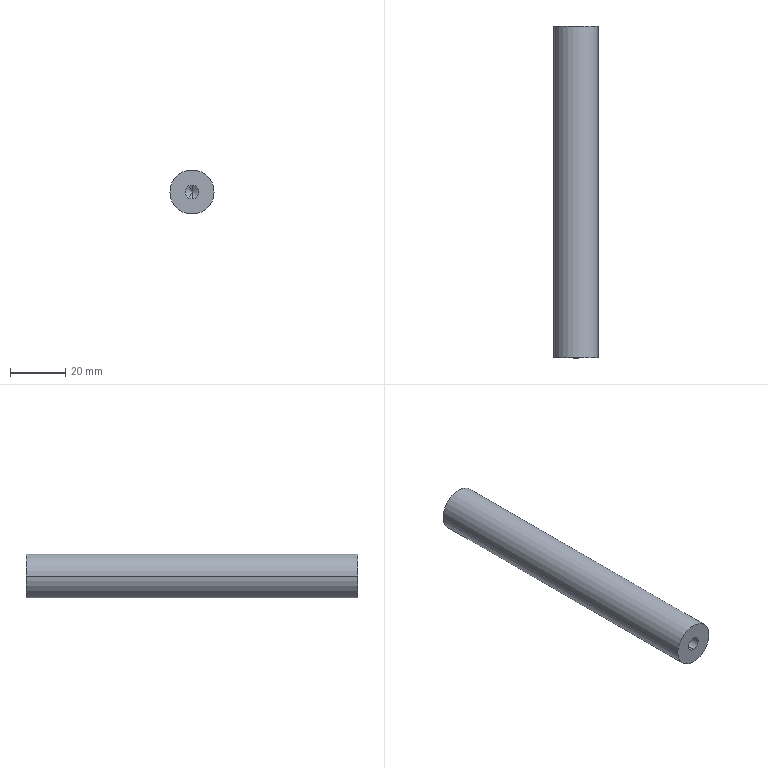Part | SolidWorks | features HoleWzd 2, RevolutionThin 1 | 1 solid | 12 faces | box 16 x 120 x 16 mm | volume 23637 mm3 | cylinder 6 | cone 4 | plane 2 | commonest cylinder face diameters 5 x4 16 x2
STEP:
#1=CARTESIAN_POINT('',(0.,-48.,2.5));
#2=VERTEX_POINT('',#1);
#3=CARTESIAN_POINT('',(0.,-48.,-2.5));
#4=VERTEX_POINT('',#3);
#5=CARTESIAN_POINT('',(0.,-48.,0.));
#6=DIRECTION('',(0.,-1.,0.));
#7=DIRECTION('',(0.,0.,-1.));
#8=AXIS2_PLACEMENT_3D('',#5,#6,#7);
#9=CIRCLE('',#8,2.5);
#10=EDGE_CURVE('',#2,#4,#9,.T.);
#11=ORIENTED_EDGE('',*,*,#10,.F.);
#12=CARTESIAN_POINT('',(0.,-60.,2.5));
#13=VERTEX_POINT('',#12);
#14=CARTESIAN_POINT('',(0.,-60.,2.5));
#15=DIRECTION('',(0.,-1.,0.));
#16=VECTOR('',#15,1000.);
#17=LINE('',#14,#16);
#18=EDGE_CURVE('',#2,#13,#17,.T.);
#19=ORIENTED_EDGE('',*,*,#18,.T.);
#20=CARTESIAN_POINT('',(0.,-60.,-2.5));
#21=VERTEX_POINT('',#20);
#22=CARTESIAN_POINT('',(0.,-60.,0.));
#23=DIRECTION('',(0.,-1.,0.));
#24=DIRECTION('',(0.,0.,-1.));
#25=AXIS2_PLACEMENT_3D('',#22,#23,#24);
#26=CIRCLE('',#25,2.5);
#27=EDGE_CURVE('',#13,#21,#26,.T.);
#28=ORIENTED_EDGE('',*,*,#27,.T.);
#29=CARTESIAN_POINT('',(0.,-60.,-2.5));
#30=DIRECTION('',(0.,-1.,0.));
#31=VECTOR('',#30,1000.);
#32=LINE('',#29,#31);
#33=EDGE_CURVE('',#4,#21,#32,.T.);
#34=ORIENTED_EDGE('',*,*,#33,.F.);
#35=EDGE_LOOP('',(#11,#19,#28,#34));
#36=FACE_OUTER_BOUND('',#35,.T.);
#37=CARTESIAN_POINT('',(0.,-60.,0.));
#38=DIRECTION('',(0.,-1.,0.));
#39=DIRECTION('',(0.,0.,-1.));
#40=AXIS2_PLACEMENT_3D('',#37,#38,#39);
#41=CYLINDRICAL_SURFACE('',#40,2.5);
#42=ADVANCED_FACE('',(#36),#41,.F.);
#43=CARTESIAN_POINT('',(0.,-46.498,0.));
#44=VERTEX_POINT('',#43);
#45=CARTESIAN_POINT('',(0.,-48.,-2.5));
#46=DIRECTION('',(0.,-0.515,-0.8572));
#47=VECTOR('',#46,1000.);
#48=LINE('',#45,#47);
#49=EDGE_CURVE('',#44,#4,#48,.T.);
#50=ORIENTED_EDGE('',*,*,#49,.F.);
#51=CARTESIAN_POINT('',(0.,-48.,2.5));
#52=DIRECTION('',(0.,-0.515,0.8572));
#53=VECTOR('',#52,1000.);
#54=LINE('',#51,#53);
#55=EDGE_CURVE('',#44,#2,#54,.T.);
#56=ORIENTED_EDGE('',*,*,#55,.T.);
#57=ORIENTED_EDGE('',*,*,#10,.T.);
#58=EDGE_LOOP('',(#50,#56,#57));
#59=FACE_OUTER_BOUND('',#58,.T.);
#60=CARTESIAN_POINT('',(0.,-48.,0.));
#61=DIRECTION('',(0.,-1.,0.));
#62=DIRECTION('',(0.,0.,-1.));
#63=AXIS2_PLACEMENT_3D('',#60,#61,#62);
#64=CONICAL_SURFACE('',#63,2.5,1.03);
#65=ADVANCED_FACE('',(#59),#64,.F.);
#66=CARTESIAN_POINT('',(0.,48.,-2.5));
#67=VERTEX_POINT('',#66);
#68=CARTESIAN_POINT('',(0.,48.,2.5));
#69=VERTEX_POINT('',#68);
#70=CARTESIAN_POINT('',(0.,48.,0.));
#71=DIRECTION('',(0.,1.,0.));
#72=DIRECTION('',(0.,0.,1.));
#73=AXIS2_PLACEMENT_3D('',#70,#71,#72);
#74=CIRCLE('',#73,2.5);
#75=EDGE_CURVE('',#67,#69,#74,.T.);
#76=ORIENTED_EDGE('',*,*,#75,.F.);
#77=CARTESIAN_POINT('',(0.,60.,-2.5));
#78=VERTEX_POINT('',#77);
#79=CARTESIAN_POINT('',(0.,60.,-2.5));
#80=DIRECTION('',(0.,1.,0.));
#81=VECTOR('',#80,1000.);
#82=LINE('',#79,#81);
#83=EDGE_CURVE('',#67,#78,#82,.T.);
#84=ORIENTED_EDGE('',*,*,#83,.T.);
#85=CARTESIAN_POINT('',(0.,60.,2.5));
#86=VERTEX_POINT('',#85);
#87=CARTESIAN_POINT('',(0.,60.,0.));
#88=DIRECTION('',(0.,1.,0.));
#89=DIRECTION('',(0.,0.,1.));
#90=AXIS2_PLACEMENT_3D('',#87,#88,#89);
#91=CIRCLE('',#90,2.5);
#92=EDGE_CURVE('',#78,#86,#91,.T.);
#93=ORIENTED_EDGE('',*,*,#92,.T.);
#94=CARTESIAN_POINT('',(0.,60.,2.5));
#95=DIRECTION('',(0.,1.,0.));
#96=VECTOR('',#95,1000.);
#97=LINE('',#94,#96);
#98=EDGE_CURVE('',#69,#86,#97,.T.);
#99=ORIENTED_EDGE('',*,*,#98,.F.);
#100=EDGE_LOOP('',(#76,#84,#93,#99));
#101=FACE_OUTER_BOUND('',#100,.T.);
#102=CARTESIAN_POINT('',(0.,60.,0.));
#103=DIRECTION('',(0.,1.,0.));
#104=DIRECTION('',(0.,0.,1.));
#105=AXIS2_PLACEMENT_3D('',#102,#103,#104);
#106=CYLINDRICAL_SURFACE('',#105,2.5);
#107=ADVANCED_FACE('',(#101),#106,.F.);
#108=CARTESIAN_POINT('',(0.,46.498,0.));
#109=VERTEX_POINT('',#108);
#110=CARTESIAN_POINT('',(0.,48.,2.5));
#111=DIRECTION('',(0.,0.515,0.8572));
#112=VECTOR('',#111,1000.);
#113=LINE('',#110,#112);
#114=EDGE_CURVE('',#109,#69,#113,.T.);
#115=ORIENTED_EDGE('',*,*,#114,.F.);
#116=CARTESIAN_POINT('',(0.,48.,-2.5));
#117=DIRECTION('',(0.,0.515,-0.8572));
#118=VECTOR('',#117,1000.);
#119=LINE('',#116,#118);
#120=EDGE_CURVE('',#109,#67,#119,.T.);
#121=ORIENTED_EDGE('',*,*,#120,.T.);
#122=ORIENTED_EDGE('',*,*,#75,.T.);
#123=EDGE_LOOP('',(#115,#121,#122));
#124=FACE_OUTER_BOUND('',#123,.T.);
#125=CARTESIAN_POINT('',(0.,48.,0.));
#126=DIRECTION('',(0.,1.,0.));
#127=DIRECTION('',(0.,0.,1.));
#128=AXIS2_PLACEMENT_3D('',#125,#126,#127);
#129=CONICAL_SURFACE('',#128,2.5,1.03);
#130=ADVANCED_FACE('',(#124),#129,.F.);
#131=CARTESIAN_POINT('',(-8.,-60.,0.));
#132=VERTEX_POINT('',#131);
#133=CARTESIAN_POINT('',(8.,-60.,0.));
#134=VERTEX_POINT('',#133);
#135=CARTESIAN_POINT('',(0.,-60.,0.));
#136=DIRECTION('',(0.,1.,0.));
#137=DIRECTION('',(-1.,0.,0.));
#138=AXIS2_PLACEMENT_3D('',#135,#136,#137);
#139=CIRCLE('',#138,8.);
#140=EDGE_CURVE('',#132,#134,#139,.T.);
#141=ORIENTED_EDGE('',*,*,#140,.T.);
#142=CARTESIAN_POINT('',(8.,60.,0.));
#143=VERTEX_POINT('',#142);
#144=CARTESIAN_POINT('',(8.,60.,0.));
#145=DIRECTION('',(0.,1.,0.));
#146=VECTOR('',#145,1000.);
#147=LINE('',#144,#146);
#148=EDGE_CURVE('',#134,#143,#147,.T.);
#149=ORIENTED_EDGE('',*,*,#148,.T.);
#150=CARTESIAN_POINT('',(-8.,60.,0.));
#151=VERTEX_POINT('',#150);
#152=CARTESIAN_POINT('',(0.,60.,0.));
#153=DIRECTION('',(0.,1.,0.));
#154=DIRECTION('',(-1.,0.,0.));
#155=AXIS2_PLACEMENT_3D('',#152,#153,#154);
#156=CIRCLE('',#155,8.);
#157=EDGE_CURVE('',#151,#143,#156,.T.);
#158=ORIENTED_EDGE('',*,*,#157,.F.);
#159=CARTESIAN_POINT('',(-8.,60.,0.));
#160=DIRECTION('',(0.,1.,0.));
#161=VECTOR('',#160,1000.);
#162=LINE('',#159,#161);
#163=EDGE_CURVE('',#132,#151,#162,.T.);
#164=ORIENTED_EDGE('',*,*,#163,.F.);
#165=EDGE_LOOP('',(#141,#149,#158,#164));
#166=FACE_OUTER_BOUND('',#165,.T.);
#167=CARTESIAN_POINT('',(0.,60.,0.));
#168=DIRECTION('',(0.,1.,0.));
#169=DIRECTION('',(-1.,0.,0.));
#170=AXIS2_PLACEMENT_3D('',#167,#168,#169);
#171=CYLINDRICAL_SURFACE('',#170,8.);
#172=ADVANCED_FACE('',(#166),#171,.T.);
#173=ORIENTED_EDGE('',*,*,#148,.F.);
#174=CARTESIAN_POINT('',(0.,-60.,0.));
#175=DIRECTION('',(0.,1.,0.));
#176=DIRECTION('',(-1.,0.,0.));
#177=AXIS2_PLACEMENT_3D('',#174,#175,#176);
#178=CIRCLE('',#177,8.);
#179=EDGE_CURVE('',#134,#132,#178,.T.);
#180=ORIENTED_EDGE('',*,*,#179,.T.);
#181=ORIENTED_EDGE('',*,*,#163,.T.);
#182=CARTESIAN_POINT('',(0.,60.,0.));
#183=DIRECTION('',(0.,1.,0.));
#184=DIRECTION('',(-1.,0.,0.));
#185=AXIS2_PLACEMENT_3D('',#182,#183,#184);
#186=CIRCLE('',#185,8.);
#187=EDGE_CURVE('',#143,#151,#186,.T.);
#188=ORIENTED_EDGE('',*,*,#187,.F.);
#189=EDGE_LOOP('',(#173,#180,#181,#188));
#190=FACE_OUTER_BOUND('',#189,.T.);
#191=CARTESIAN_POINT('',(0.,60.,0.));
#192=DIRECTION('',(0.,1.,0.));
#193=DIRECTION('',(-1.,0.,0.));
#194=AXIS2_PLACEMENT_3D('',#191,#192,#193);
#195=CYLINDRICAL_SURFACE('',#194,8.);
#196=ADVANCED_FACE('',(#190),#195,.T.);
#197=CARTESIAN_POINT('',(0.,60.,0.));
#198=DIRECTION('',(0.,1.,0.));
#199=DIRECTION('',(0.,0.,1.));
#200=AXIS2_PLACEMENT_3D('',#197,#198,#199);
#201=CIRCLE('',#200,2.5);
#202=EDGE_CURVE('',#86,#78,#201,.T.);
#203=ORIENTED_EDGE('',*,*,#202,.F.);
#204=ORIENTED_EDGE('',*,*,#92,.F.);
#205=EDGE_LOOP('',(#203,#204));
#206=FACE_BOUND('',#205,.T.);
#207=ORIENTED_EDGE('',*,*,#157,.T.);
#208=ORIENTED_EDGE('',*,*,#187,.T.);
#209=EDGE_LOOP('',(#207,#208));
#210=FACE_OUTER_BOUND('',#209,.T.);
#211=CARTESIAN_POINT('',(-8.,60.,0.));
#212=DIRECTION('',(0.,-1.,0.));
#213=DIRECTION('',(1.,0.,0.));
#214=AXIS2_PLACEMENT_3D('',#211,#212,#213);
#215=PLANE('',#214);
#216=ADVANCED_FACE('',(#206,#210),#215,.F.);
#217=CARTESIAN_POINT('',(0.,-60.,0.));
#218=DIRECTION('',(0.,-1.,0.));
#219=DIRECTION('',(0.,0.,-1.));
#220=AXIS2_PLACEMENT_3D('',#217,#218,#219);
#221=CIRCLE('',#220,2.5);
#222=EDGE_CURVE('',#21,#13,#221,.T.);
#223=ORIENTED_EDGE('',*,*,#222,.F.);
#224=ORIENTED_EDGE('',*,*,#27,.F.);
#225=EDGE_LOOP('',(#223,#224));
#226=FACE_BOUND('',#225,.T.);
#227=ORIENTED_EDGE('',*,*,#140,.F.);
#228=ORIENTED_EDGE('',*,*,#179,.F.);
#229=EDGE_LOOP('',(#227,#228));
#230=FACE_OUTER_BOUND('',#229,.T.);
#231=CARTESIAN_POINT('',(0.,-60.,0.));
#232=DIRECTION('',(0.,1.,0.));
#233=DIRECTION('',(-1.,0.,0.));
#234=AXIS2_PLACEMENT_3D('',#231,#232,#233);
#235=PLANE('',#234);
#236=ADVANCED_FACE('',(#226,#230),#235,.F.);
#237=ORIENTED_EDGE('',*,*,#120,.F.);
#238=ORIENTED_EDGE('',*,*,#114,.T.);
#239=CARTESIAN_POINT('',(0.,48.,0.));
#240=DIRECTION('',(0.,1.,0.));
#241=DIRECTION('',(0.,0.,1.));
#242=AXIS2_PLACEMENT_3D('',#239,#240,#241);
#243=CIRCLE('',#242,2.5);
#244=EDGE_CURVE('',#69,#67,#243,.T.);
#245=ORIENTED_EDGE('',*,*,#244,.T.);
#246=EDGE_LOOP('',(#237,#238,#245));
#247=FACE_OUTER_BOUND('',#246,.T.);
#248=CARTESIAN_POINT('',(0.,48.,0.));
#249=DIRECTION('',(0.,1.,0.));
#250=DIRECTION('',(0.,0.,1.));
#251=AXIS2_PLACEMENT_3D('',#248,#249,#250);
#252=CONICAL_SURFACE('',#251,2.5,1.03);
#253=ADVANCED_FACE('',(#247),#252,.F.);
#254=ORIENTED_EDGE('',*,*,#83,.F.);
#255=ORIENTED_EDGE('',*,*,#244,.F.);
#256=ORIENTED_EDGE('',*,*,#98,.T.);
#257=ORIENTED_EDGE('',*,*,#202,.T.);
#258=EDGE_LOOP('',(#254,#255,#256,#257));
#259=FACE_OUTER_BOUND('',#258,.T.);
#260=CARTESIAN_POINT('',(0.,60.,0.));
#261=DIRECTION('',(0.,1.,0.));
#262=DIRECTION('',(0.,0.,1.));
#263=AXIS2_PLACEMENT_3D('',#260,#261,#262);
#264=CYLINDRICAL_SURFACE('',#263,2.5);
#265=ADVANCED_FACE('',(#259),#264,.F.);
#266=ORIENTED_EDGE('',*,*,#55,.F.);
#267=ORIENTED_EDGE('',*,*,#49,.T.);
#268=CARTESIAN_POINT('',(0.,-48.,0.));
#269=DIRECTION('',(0.,-1.,0.));
#270=DIRECTION('',(0.,0.,-1.));
#271=AXIS2_PLACEMENT_3D('',#268,#269,#270);
#272=CIRCLE('',#271,2.5);
#273=EDGE_CURVE('',#4,#2,#272,.T.);
#274=ORIENTED_EDGE('',*,*,#273,.T.);
#275=EDGE_LOOP('',(#266,#267,#274));
#276=FACE_OUTER_BOUND('',#275,.T.);
#277=CARTESIAN_POINT('',(0.,-48.,0.));
#278=DIRECTION('',(0.,-1.,0.));
#279=DIRECTION('',(0.,0.,-1.));
#280=AXIS2_PLACEMENT_3D('',#277,#278,#279);
#281=CONICAL_SURFACE('',#280,2.5,1.03);
#282=ADVANCED_FACE('',(#276),#281,.F.);
#283=ORIENTED_EDGE('',*,*,#18,.F.);
#284=ORIENTED_EDGE('',*,*,#273,.F.);
#285=ORIENTED_EDGE('',*,*,#33,.T.);
#286=ORIENTED_EDGE('',*,*,#222,.T.);
#287=EDGE_LOOP('',(#283,#284,#285,#286));
#288=FACE_OUTER_BOUND('',#287,.T.);
#289=CARTESIAN_POINT('',(0.,-60.,0.));
#290=DIRECTION('',(0.,-1.,0.));
#291=DIRECTION('',(0.,0.,-1.));
#292=AXIS2_PLACEMENT_3D('',#289,#290,#291);
#293=CYLINDRICAL_SURFACE('',#292,2.5);
#294=ADVANCED_FACE('',(#288),#293,.F.);
#295=CLOSED_SHELL('',(#42,#65,#107,#130,#172,#196,#216,#236,#253,#265,#282,#294));
#296=MANIFOLD_SOLID_BREP('',#295);
#297=CARTESIAN_POINT('',(0.,0.,0.));
#298=DIRECTION('',(0.,0.,1.));
#299=DIRECTION('',(1.,0.,0.));
#300=AXIS2_PLACEMENT_3D('',#297,#298,#299);
#301=(LENGTH_UNIT()NAMED_UNIT(*)SI_UNIT(.MILLI.,.METRE.));
#302=UNCERTAINTY_MEASURE_WITH_UNIT(LENGTH_MEASURE(0.00001),#301,'','');
#303=(NAMED_UNIT(*)PLANE_ANGLE_UNIT()SI_UNIT($,.RADIAN.));
#304=(NAMED_UNIT(*)SI_UNIT($,.STERADIAN.)SOLID_ANGLE_UNIT());
#305=(GEOMETRIC_REPRESENTATION_CONTEXT(3)GLOBAL_UNCERTAINTY_ASSIGNED_CONTEXT((#302))GLOBAL_UNIT_ASSIGNED_CONTEXT((#301,#303,#304))REPRESENTATION_CONTEXT('',''));
#306=ADVANCED_BREP_SHAPE_REPRESENTATION('',(#296,#300),#305);